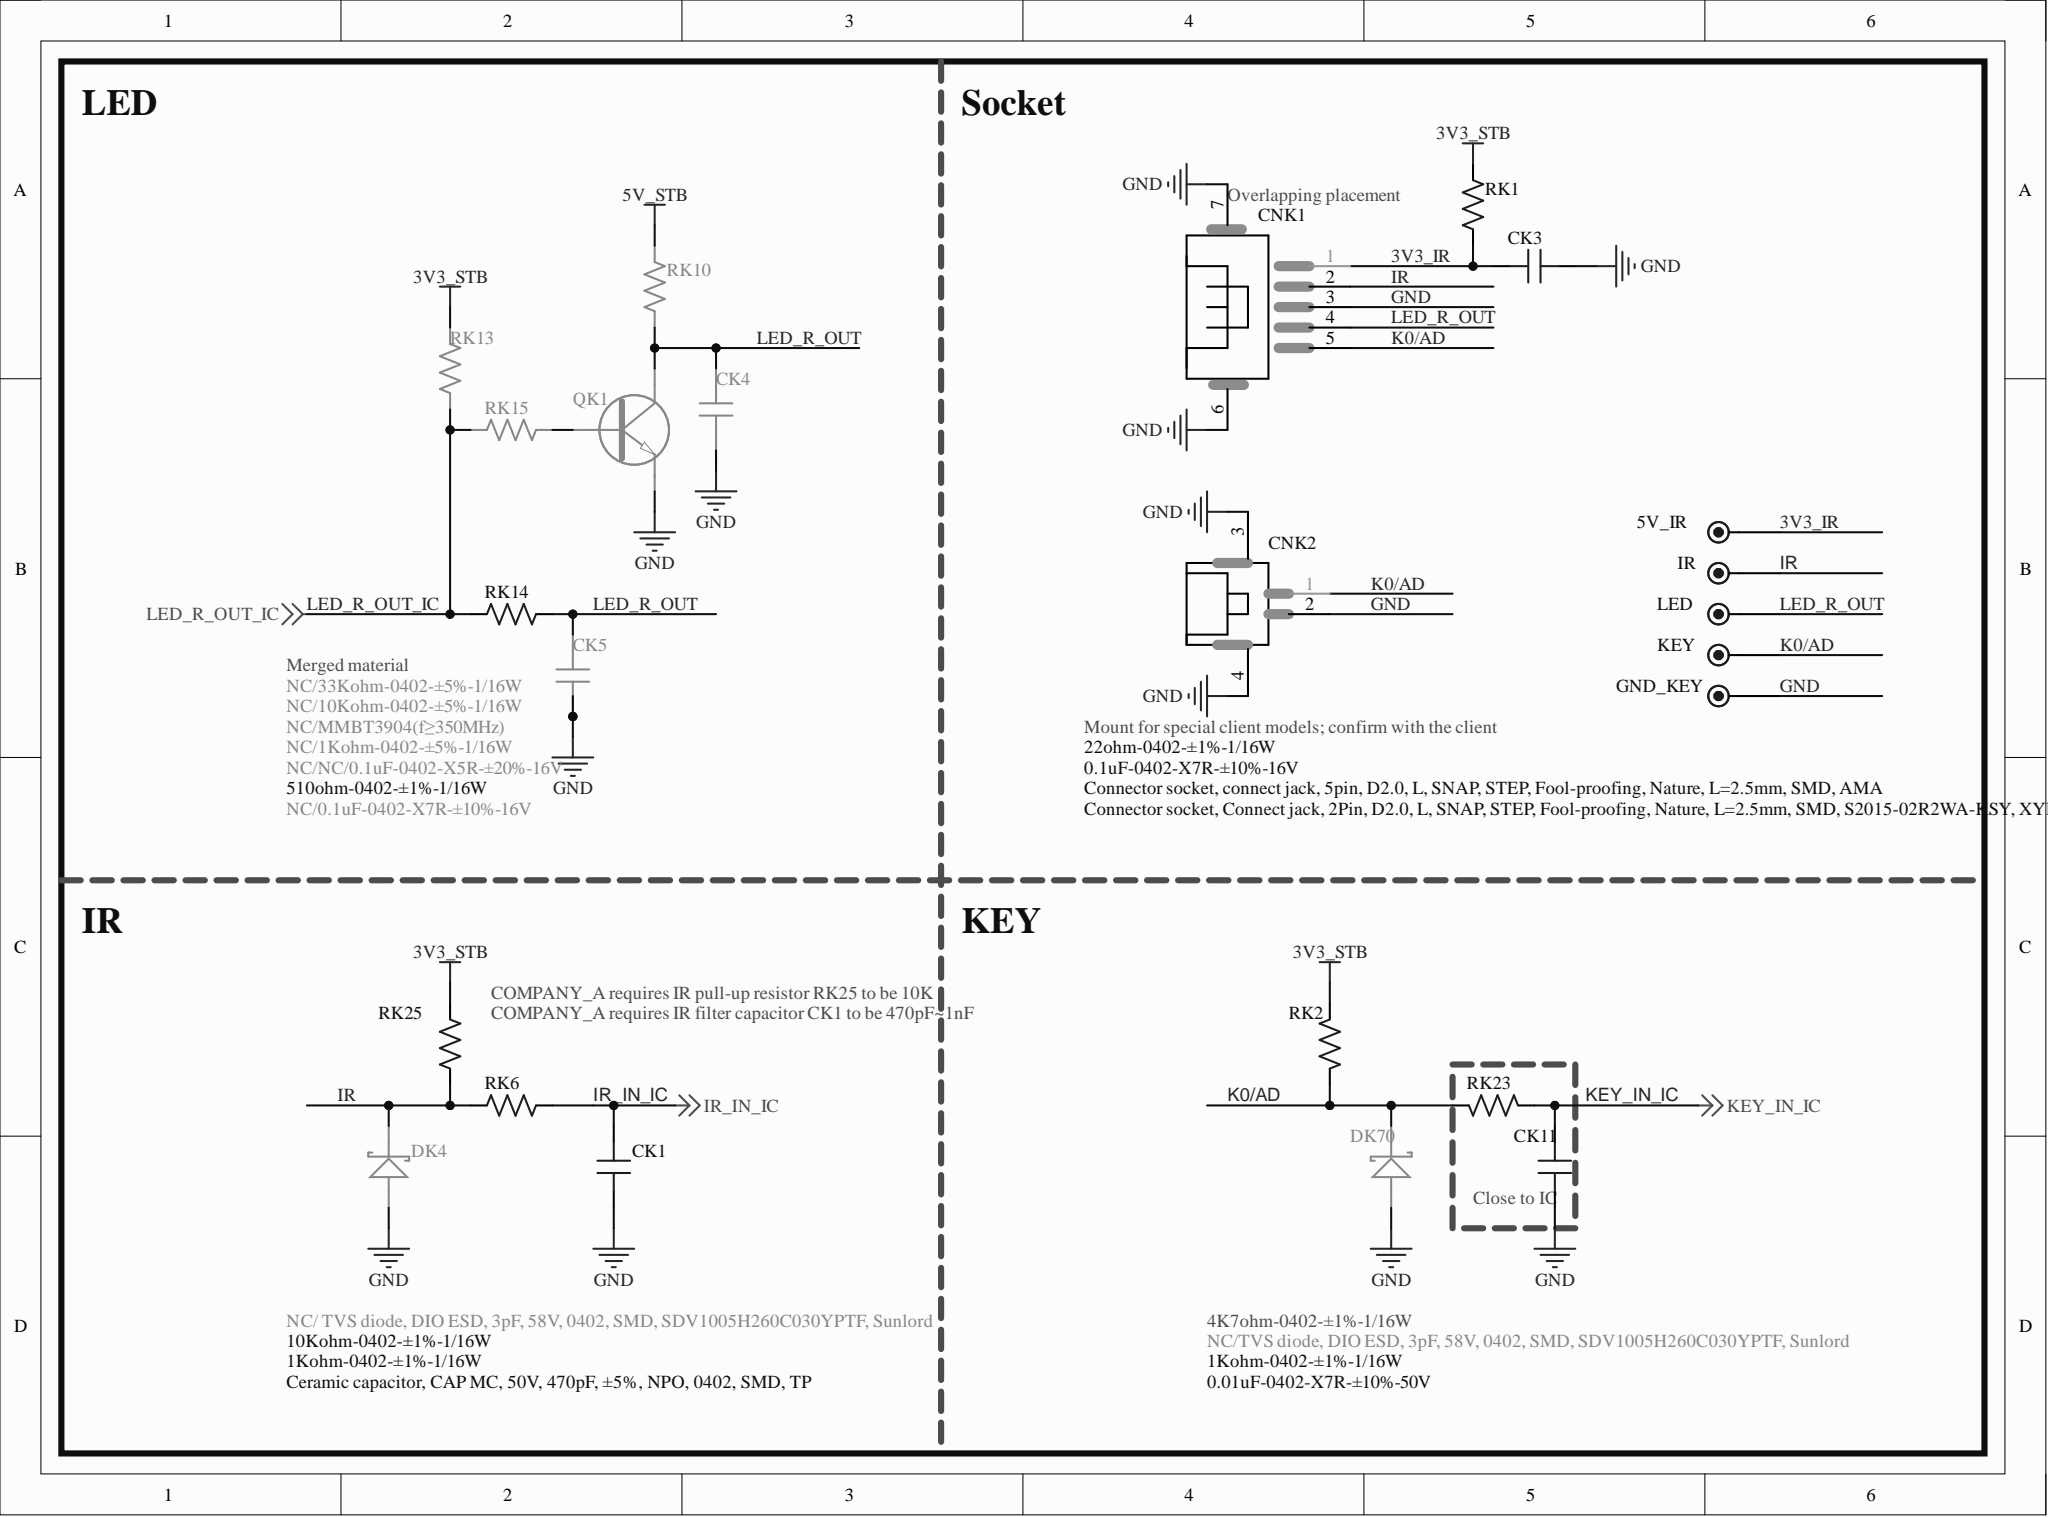Circuit board | Altium Designer | 541 parts | 263 nets | one sheet of the schematic
Parts on this sheet (reference | value | footprint):
5V_IR | DM0 | TP
CK1 | Ceramic capacitor, CAP MC, 50V, 470pF, ±5%, NPO, 0402, SMD, TP | C0402
CK3 | 0.1uF-0402-X7R-±10%-16V | C0402
CK4 | NC/NC/0.1uF-0402-X5R-±20%-16V | C0402
CK5 | NC/0.1uF-0402-X7R-±10%-16V | C0402
CK11 | 0.01uF-0402-X7R-±10%-50V | C0402
CNK1 | Connector socket, connect jack, 5pin, D2.0, L, SNAP, STEP, Fool-proofing, Nature, L=2.5mm, SMD, AMA | SIP5H/2.0S-4
CNK2 | Connector socket, Connect jack, 2Pin, D2.0, L, SNAP, STEP, Fool-proofing, Nature, L=2.5mm, SMD, S2015-02R2WA-KSY, XYDT | SIP2H/2.0S-3
DK4 | NC/ TVS diode, DIO ESD, 3pF, 58V, 0402, SMD, SDV1005H260C030YPTF, Sunlord | DIODE-S0402
DK70 | NC/TVS diode, DIO ESD, 3pF, 58V, 0402, SMD, SDV1005H260C030YPTF, Sunlord | DIODE-S0402
GND_KEY | DM0 | TP
KEY | DM0 | TP
LED | DM0 | TP
QK1 | NC/MMBT3904(f=350MHz) | SOT-23
RK1 | 22ohm-0402-±1%-1/16W | R0402
RK2 | 4K7ohm-0402-±1%-1/16W | R0402
RK6 | 1Kohm-0402-±1%-1/16W | R0402
RK10 | NC/1Kohm-0402-±5%-1/16W | R0402
RK13 | NC/33Kohm-0402-±5%-1/16W | R0402
RK14 | 510ohm-0402-±1%-1/16W | R0402
RK15 | NC/10Kohm-0402-±5%-1/16W | R0402
RK23 | 1Kohm-0402-±1%-1/16W | R0402
RK25 | 10Kohm-0402-±1%-1/16W | R0402
Nets of these parts (net: part-pin ...):
NetQK1_B: QK1-B RK15-2
LED_R_OUT_IC: RK13-1 RK14-1 RK15-1
LED_R_OUT: CK4-2 CK5-2 CNK1-4 LED-1 QK1-C RK10-1 RK14-2
KEY_IN_IC: CK11-1 RK23-1
K0/AD: CNK1-5 CNK2-1 DK70-K KEY-1 RK2-1 RK23-2
IR_IN_IC: CK1-2 RK6-2
IR: CNK1-2 DK4-K RK6-1 RK25-1
GND: CK1-1 CK3-2 CK4-1 CK5-1 CK11-2 CNK1-3 CNK1-6 CNK1-7 CNK2-2 CNK2-3 CNK2-4 DK4-A DK70-A GND_KEY-1 QK1-E
5V_STB: RK10-2
3V3_STB: RK1-1 RK2-2 RK13-2 RK25-2
3V3_IR: 5V_IR-1 CK3-1 CNK1-1 RK1-2